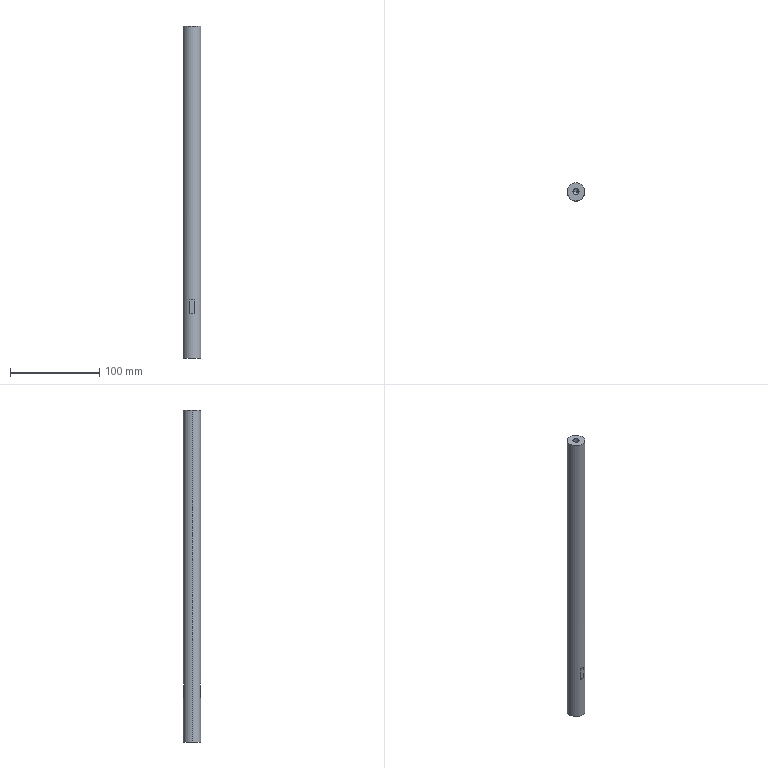Part | SolidWorks | features HoleWzd 2, Extrusion 1, ICE 1 | 1 solid | 18 faces | box 20 x 20 x 372 mm | volume 115321 mm3 | plane 8 | cylinder 6 | cone 4 | commonest cylinder face diameters 6.8 x4 20 x2
STEP:
#1=CARTESIAN_POINT('',(-3.4,0.,166.25));
#2=VERTEX_POINT('',#1);
#3=CARTESIAN_POINT('',(3.4,0.,166.25));
#4=VERTEX_POINT('',#3);
#5=CARTESIAN_POINT('',(0.,0.,166.25));
#6=DIRECTION('',(0.,0.,1.));
#7=DIRECTION('',(1.,0.,0.));
#8=AXIS2_PLACEMENT_3D('',#5,#6,#7);
#9=CIRCLE('',#8,3.4);
#10=EDGE_CURVE('',#2,#4,#9,.T.);
#11=ORIENTED_EDGE('',*,*,#10,.F.);
#12=CARTESIAN_POINT('',(-3.4,0.,186.));
#13=VERTEX_POINT('',#12);
#14=CARTESIAN_POINT('',(-3.4,0.,186.));
#15=DIRECTION('',(0.,0.,1.));
#16=VECTOR('',#15,1000.);
#17=LINE('',#14,#16);
#18=EDGE_CURVE('',#2,#13,#17,.T.);
#19=ORIENTED_EDGE('',*,*,#18,.T.);
#20=CARTESIAN_POINT('',(3.4,0.,186.));
#21=VERTEX_POINT('',#20);
#22=CARTESIAN_POINT('',(0.,0.,186.));
#23=DIRECTION('',(0.,0.,1.));
#24=DIRECTION('',(1.,0.,0.));
#25=AXIS2_PLACEMENT_3D('',#22,#23,#24);
#26=CIRCLE('',#25,3.4);
#27=EDGE_CURVE('',#13,#21,#26,.T.);
#28=ORIENTED_EDGE('',*,*,#27,.T.);
#29=CARTESIAN_POINT('',(3.4,0.,186.));
#30=DIRECTION('',(0.,0.,1.));
#31=VECTOR('',#30,1000.);
#32=LINE('',#29,#31);
#33=EDGE_CURVE('',#4,#21,#32,.T.);
#34=ORIENTED_EDGE('',*,*,#33,.F.);
#35=EDGE_LOOP('',(#11,#19,#28,#34));
#36=FACE_OUTER_BOUND('',#35,.T.);
#37=CARTESIAN_POINT('',(0.,0.,186.));
#38=DIRECTION('',(0.,0.,1.));
#39=DIRECTION('',(1.,0.,0.));
#40=AXIS2_PLACEMENT_3D('',#37,#38,#39);
#41=CYLINDRICAL_SURFACE('',#40,3.4);
#42=ADVANCED_FACE('',(#36),#41,.F.);
#43=CARTESIAN_POINT('',(0.,0.,164.207));
#44=VERTEX_POINT('',#43);
#45=CARTESIAN_POINT('',(3.4,0.,166.25));
#46=DIRECTION('',(0.8572,0.,0.515));
#47=VECTOR('',#46,1000.);
#48=LINE('',#45,#47);
#49=EDGE_CURVE('',#44,#4,#48,.T.);
#50=ORIENTED_EDGE('',*,*,#49,.F.);
#51=CARTESIAN_POINT('',(-3.4,0.,166.25));
#52=DIRECTION('',(-0.8572,0.,0.515));
#53=VECTOR('',#52,1000.);
#54=LINE('',#51,#53);
#55=EDGE_CURVE('',#44,#2,#54,.T.);
#56=ORIENTED_EDGE('',*,*,#55,.T.);
#57=ORIENTED_EDGE('',*,*,#10,.T.);
#58=EDGE_LOOP('',(#50,#56,#57));
#59=FACE_OUTER_BOUND('',#58,.T.);
#60=CARTESIAN_POINT('',(0.,0.,166.25));
#61=DIRECTION('',(0.,0.,1.));
#62=DIRECTION('',(1.,0.,0.));
#63=AXIS2_PLACEMENT_3D('',#60,#61,#62);
#64=CONICAL_SURFACE('',#63,3.4,1.03);
#65=ADVANCED_FACE('',(#59),#64,.F.);
#66=CARTESIAN_POINT('',(3.4,0.,-166.25));
#67=VERTEX_POINT('',#66);
#68=CARTESIAN_POINT('',(-3.4,0.,-166.25));
#69=VERTEX_POINT('',#68);
#70=CARTESIAN_POINT('',(0.,0.,-166.25));
#71=DIRECTION('',(0.,0.,-1.));
#72=DIRECTION('',(-1.,0.,0.));
#73=AXIS2_PLACEMENT_3D('',#70,#71,#72);
#74=CIRCLE('',#73,3.4);
#75=EDGE_CURVE('',#67,#69,#74,.T.);
#76=ORIENTED_EDGE('',*,*,#75,.F.);
#77=CARTESIAN_POINT('',(3.4,0.,-186.));
#78=VERTEX_POINT('',#77);
#79=CARTESIAN_POINT('',(3.4,0.,-186.));
#80=DIRECTION('',(0.,0.,-1.));
#81=VECTOR('',#80,1000.);
#82=LINE('',#79,#81);
#83=EDGE_CURVE('',#67,#78,#82,.T.);
#84=ORIENTED_EDGE('',*,*,#83,.T.);
#85=CARTESIAN_POINT('',(-3.4,0.,-186.));
#86=VERTEX_POINT('',#85);
#87=CARTESIAN_POINT('',(0.,0.,-186.));
#88=DIRECTION('',(0.,0.,-1.));
#89=DIRECTION('',(-1.,0.,0.));
#90=AXIS2_PLACEMENT_3D('',#87,#88,#89);
#91=CIRCLE('',#90,3.4);
#92=EDGE_CURVE('',#78,#86,#91,.T.);
#93=ORIENTED_EDGE('',*,*,#92,.T.);
#94=CARTESIAN_POINT('',(-3.4,0.,-186.));
#95=DIRECTION('',(0.,0.,-1.));
#96=VECTOR('',#95,1000.);
#97=LINE('',#94,#96);
#98=EDGE_CURVE('',#69,#86,#97,.T.);
#99=ORIENTED_EDGE('',*,*,#98,.F.);
#100=EDGE_LOOP('',(#76,#84,#93,#99));
#101=FACE_OUTER_BOUND('',#100,.T.);
#102=CARTESIAN_POINT('',(0.,0.,-186.));
#103=DIRECTION('',(0.,0.,-1.));
#104=DIRECTION('',(-1.,0.,0.));
#105=AXIS2_PLACEMENT_3D('',#102,#103,#104);
#106=CYLINDRICAL_SURFACE('',#105,3.4);
#107=ADVANCED_FACE('',(#101),#106,.F.);
#108=CARTESIAN_POINT('',(0.,0.,-164.207));
#109=VERTEX_POINT('',#108);
#110=CARTESIAN_POINT('',(-3.4,0.,-166.25));
#111=DIRECTION('',(-0.8572,0.,-0.515));
#112=VECTOR('',#111,1000.);
#113=LINE('',#110,#112);
#114=EDGE_CURVE('',#109,#69,#113,.T.);
#115=ORIENTED_EDGE('',*,*,#114,.F.);
#116=CARTESIAN_POINT('',(3.4,0.,-166.25));
#117=DIRECTION('',(0.8572,0.,-0.515));
#118=VECTOR('',#117,1000.);
#119=LINE('',#116,#118);
#120=EDGE_CURVE('',#109,#67,#119,.T.);
#121=ORIENTED_EDGE('',*,*,#120,.T.);
#122=ORIENTED_EDGE('',*,*,#75,.T.);
#123=EDGE_LOOP('',(#115,#121,#122));
#124=FACE_OUTER_BOUND('',#123,.T.);
#125=CARTESIAN_POINT('',(0.,0.,-166.25));
#126=DIRECTION('',(0.,0.,-1.));
#127=DIRECTION('',(-1.,0.,0.));
#128=AXIS2_PLACEMENT_3D('',#125,#126,#127);
#129=CONICAL_SURFACE('',#128,3.4,1.03);
#130=ADVANCED_FACE('',(#124),#129,.F.);
#131=CARTESIAN_POINT('',(-3.122,9.5,-136.));
#132=VERTEX_POINT('',#131);
#133=CARTESIAN_POINT('',(-3.122,9.5,-121.));
#134=VERTEX_POINT('',#133);
#135=CARTESIAN_POINT('',(-3.122,9.5,-136.));
#136=DIRECTION('',(0.,0.,1.));
#137=VECTOR('',#136,1000.);
#138=LINE('',#135,#137);
#139=EDGE_CURVE('',#132,#134,#138,.T.);
#140=ORIENTED_EDGE('',*,*,#139,.F.);
#141=CARTESIAN_POINT('',(3.122,9.5,-136.));
#142=VERTEX_POINT('',#141);
#143=CARTESIAN_POINT('',(0.,0.,-136.));
#144=DIRECTION('',(0.,0.,-1.));
#145=DIRECTION('',(-1.,0.,0.));
#146=AXIS2_PLACEMENT_3D('',#143,#144,#145);
#147=CIRCLE('',#146,10.);
#148=EDGE_CURVE('',#132,#142,#147,.T.);
#149=ORIENTED_EDGE('',*,*,#148,.T.);
#150=CARTESIAN_POINT('',(3.122,9.5,-121.));
#151=VERTEX_POINT('',#150);
#152=CARTESIAN_POINT('',(3.122,9.5,-136.));
#153=DIRECTION('',(0.,0.,1.));
#154=VECTOR('',#153,1000.);
#155=LINE('',#152,#154);
#156=EDGE_CURVE('',#142,#151,#155,.T.);
#157=ORIENTED_EDGE('',*,*,#156,.T.);
#158=CARTESIAN_POINT('',(0.,0.,-121.));
#159=DIRECTION('',(0.,0.,-1.));
#160=DIRECTION('',(-1.,0.,0.));
#161=AXIS2_PLACEMENT_3D('',#158,#159,#160);
#162=CIRCLE('',#161,10.);
#163=EDGE_CURVE('',#134,#151,#162,.T.);
#164=ORIENTED_EDGE('',*,*,#163,.F.);
#165=EDGE_LOOP('',(#140,#149,#157,#164));
#166=FACE_BOUND('',#165,.T.);
#167=CARTESIAN_POINT('',(10.,0.,186.));
#168=VERTEX_POINT('',#167);
#169=CARTESIAN_POINT('',(-10.,0.,186.));
#170=VERTEX_POINT('',#169);
#171=CARTESIAN_POINT('',(0.,0.,186.));
#172=DIRECTION('',(0.,0.,1.));
#173=DIRECTION('',(1.,0.,0.));
#174=AXIS2_PLACEMENT_3D('',#171,#172,#173);
#175=CIRCLE('',#174,10.);
#176=EDGE_CURVE('',#168,#170,#175,.T.);
#177=ORIENTED_EDGE('',*,*,#176,.F.);
#178=CARTESIAN_POINT('',(10.,0.,-186.));
#179=VERTEX_POINT('',#178);
#180=CARTESIAN_POINT('',(10.,0.,186.));
#181=DIRECTION('',(0.,0.,-1.));
#182=VECTOR('',#181,1000.);
#183=LINE('',#180,#182);
#184=EDGE_CURVE('',#168,#179,#183,.T.);
#185=ORIENTED_EDGE('',*,*,#184,.T.);
#186=CARTESIAN_POINT('',(-10.,0.,-186.));
#187=VERTEX_POINT('',#186);
#188=CARTESIAN_POINT('',(0.,0.,-186.));
#189=DIRECTION('',(0.,0.,1.));
#190=DIRECTION('',(1.,0.,0.));
#191=AXIS2_PLACEMENT_3D('',#188,#189,#190);
#192=CIRCLE('',#191,10.);
#193=EDGE_CURVE('',#179,#187,#192,.T.);
#194=ORIENTED_EDGE('',*,*,#193,.T.);
#195=CARTESIAN_POINT('',(-10.,0.,186.));
#196=DIRECTION('',(0.,0.,-1.));
#197=VECTOR('',#196,1000.);
#198=LINE('',#195,#197);
#199=EDGE_CURVE('',#170,#187,#198,.T.);
#200=ORIENTED_EDGE('',*,*,#199,.F.);
#201=EDGE_LOOP('',(#177,#185,#194,#200));
#202=FACE_OUTER_BOUND('',#201,.T.);
#203=CARTESIAN_POINT('',(0.,0.,186.));
#204=DIRECTION('',(0.,0.,-1.));
#205=DIRECTION('',(-1.,0.,0.));
#206=AXIS2_PLACEMENT_3D('',#203,#204,#205);
#207=CYLINDRICAL_SURFACE('',#206,10.);
#208=ADVANCED_FACE('',(#166,#202),#207,.T.);
#209=ORIENTED_EDGE('',*,*,#184,.F.);
#210=CARTESIAN_POINT('',(0.,0.,186.));
#211=DIRECTION('',(0.,0.,1.));
#212=DIRECTION('',(1.,0.,0.));
#213=AXIS2_PLACEMENT_3D('',#210,#211,#212);
#214=CIRCLE('',#213,10.);
#215=EDGE_CURVE('',#170,#168,#214,.T.);
#216=ORIENTED_EDGE('',*,*,#215,.F.);
#217=ORIENTED_EDGE('',*,*,#199,.T.);
#218=CARTESIAN_POINT('',(0.,0.,-186.));
#219=DIRECTION('',(0.,0.,1.));
#220=DIRECTION('',(1.,0.,0.));
#221=AXIS2_PLACEMENT_3D('',#218,#219,#220);
#222=CIRCLE('',#221,10.);
#223=EDGE_CURVE('',#187,#179,#222,.T.);
#224=ORIENTED_EDGE('',*,*,#223,.T.);
#225=EDGE_LOOP('',(#209,#216,#217,#224));
#226=FACE_OUTER_BOUND('',#225,.T.);
#227=CARTESIAN_POINT('',(3.122,-9.5,-136.));
#228=VERTEX_POINT('',#227);
#229=CARTESIAN_POINT('',(3.122,-9.5,-121.));
#230=VERTEX_POINT('',#229);
#231=CARTESIAN_POINT('',(3.122,-9.5,-136.));
#232=DIRECTION('',(0.,0.,1.));
#233=VECTOR('',#232,1000.);
#234=LINE('',#231,#233);
#235=EDGE_CURVE('',#228,#230,#234,.T.);
#236=ORIENTED_EDGE('',*,*,#235,.F.);
#237=CARTESIAN_POINT('',(-3.122,-9.5,-136.));
#238=VERTEX_POINT('',#237);
#239=CARTESIAN_POINT('',(0.,0.,-136.));
#240=DIRECTION('',(0.,0.,-1.));
#241=DIRECTION('',(-1.,0.,0.));
#242=AXIS2_PLACEMENT_3D('',#239,#240,#241);
#243=CIRCLE('',#242,10.);
#244=EDGE_CURVE('',#228,#238,#243,.T.);
#245=ORIENTED_EDGE('',*,*,#244,.T.);
#246=CARTESIAN_POINT('',(-3.122,-9.5,-121.));
#247=VERTEX_POINT('',#246);
#248=CARTESIAN_POINT('',(-3.122,-9.5,-136.));
#249=DIRECTION('',(0.,0.,1.));
#250=VECTOR('',#249,1000.);
#251=LINE('',#248,#250);
#252=EDGE_CURVE('',#238,#247,#251,.T.);
#253=ORIENTED_EDGE('',*,*,#252,.T.);
#254=CARTESIAN_POINT('',(0.,0.,-121.));
#255=DIRECTION('',(0.,0.,-1.));
#256=DIRECTION('',(-1.,0.,0.));
#257=AXIS2_PLACEMENT_3D('',#254,#255,#256);
#258=CIRCLE('',#257,10.);
#259=EDGE_CURVE('',#230,#247,#258,.T.);
#260=ORIENTED_EDGE('',*,*,#259,.F.);
#261=EDGE_LOOP('',(#236,#245,#253,#260));
#262=FACE_BOUND('',#261,.T.);
#263=CARTESIAN_POINT('',(0.,0.,186.));
#264=DIRECTION('',(0.,0.,-1.));
#265=DIRECTION('',(-1.,0.,0.));
#266=AXIS2_PLACEMENT_3D('',#263,#264,#265);
#267=CYLINDRICAL_SURFACE('',#266,10.);
#268=ADVANCED_FACE('',(#226,#262),#267,.T.);
#269=CARTESIAN_POINT('',(0.,0.,186.));
#270=DIRECTION('',(0.,0.,1.));
#271=DIRECTION('',(1.,0.,0.));
#272=AXIS2_PLACEMENT_3D('',#269,#270,#271);
#273=CIRCLE('',#272,3.4);
#274=EDGE_CURVE('',#21,#13,#273,.T.);
#275=ORIENTED_EDGE('',*,*,#274,.F.);
#276=ORIENTED_EDGE('',*,*,#27,.F.);
#277=EDGE_LOOP('',(#275,#276));
#278=FACE_BOUND('',#277,.T.);
#279=ORIENTED_EDGE('',*,*,#215,.T.);
#280=ORIENTED_EDGE('',*,*,#176,.T.);
#281=EDGE_LOOP('',(#279,#280));
#282=FACE_OUTER_BOUND('',#281,.T.);
#283=CARTESIAN_POINT('',(0.,0.,186.));
#284=DIRECTION('',(0.,0.,1.));
#285=DIRECTION('',(1.,0.,0.));
#286=AXIS2_PLACEMENT_3D('',#283,#284,#285);
#287=PLANE('',#286);
#288=ADVANCED_FACE('',(#278,#282),#287,.T.);
#289=CARTESIAN_POINT('',(0.,0.,-186.));
#290=DIRECTION('',(0.,0.,-1.));
#291=DIRECTION('',(-1.,0.,0.));
#292=AXIS2_PLACEMENT_3D('',#289,#290,#291);
#293=CIRCLE('',#292,3.4);
#294=EDGE_CURVE('',#86,#78,#293,.T.);
#295=ORIENTED_EDGE('',*,*,#294,.F.);
#296=ORIENTED_EDGE('',*,*,#92,.F.);
#297=EDGE_LOOP('',(#295,#296));
#298=FACE_BOUND('',#297,.T.);
#299=ORIENTED_EDGE('',*,*,#223,.F.);
#300=ORIENTED_EDGE('',*,*,#193,.F.);
#301=EDGE_LOOP('',(#299,#300));
#302=FACE_OUTER_BOUND('',#301,.T.);
#303=CARTESIAN_POINT('',(0.,0.,-186.));
#304=DIRECTION('',(0.,0.,1.));
#305=DIRECTION('',(1.,0.,0.));
#306=AXIS2_PLACEMENT_3D('',#303,#304,#305);
#307=PLANE('',#306);
#308=ADVANCED_FACE('',(#298,#302),#307,.F.);
#309=CARTESIAN_POINT('',(3.122,-9.5,-121.));
#310=DIRECTION('',(1.,0.,0.));
#311=VECTOR('',#310,1000.);
#312=LINE('',#309,#311);
#313=EDGE_CURVE('',#247,#230,#312,.T.);
#314=ORIENTED_EDGE('',*,*,#313,.F.);
#315=ORIENTED_EDGE('',*,*,#252,.F.);
#316=CARTESIAN_POINT('',(3.122,-9.5,-136.));
#317=DIRECTION('',(1.,0.,0.));
#318=VECTOR('',#317,1000.);
#319=LINE('',#316,#318);
#320=EDGE_CURVE('',#238,#228,#319,.T.);
#321=ORIENTED_EDGE('',*,*,#320,.T.);
#322=ORIENTED_EDGE('',*,*,#235,.T.);
#323=EDGE_LOOP('',(#314,#315,#321,#322));
#324=FACE_OUTER_BOUND('',#323,.T.);
#325=CARTESIAN_POINT('',(3.122,-9.5,-136.));
#326=DIRECTION('',(0.,-1.,0.));
#327=DIRECTION('',(0.,0.,-1.));
#328=AXIS2_PLACEMENT_3D('',#325,#326,#327);
#329=PLANE('',#328);
#330=ADVANCED_FACE('',(#324),#329,.T.);
#331=ORIENTED_EDGE('',*,*,#244,.F.);
#332=ORIENTED_EDGE('',*,*,#320,.F.);
#333=EDGE_LOOP('',(#331,#332));
#334=FACE_OUTER_BOUND('',#333,.T.);
#335=CARTESIAN_POINT('',(0.,0.,-136.));
#336=DIRECTION('',(0.,0.,-1.));
#337=DIRECTION('',(-1.,0.,0.));
#338=AXIS2_PLACEMENT_3D('',#335,#336,#337);
#339=PLANE('',#338);
#340=ADVANCED_FACE('',(#334),#339,.F.);
#341=ORIENTED_EDGE('',*,*,#259,.T.);
#342=ORIENTED_EDGE('',*,*,#313,.T.);
#343=EDGE_LOOP('',(#341,#342));
#344=FACE_OUTER_BOUND('',#343,.T.);
#345=CARTESIAN_POINT('',(0.,0.,-121.));
#346=DIRECTION('',(0.,0.,-1.));
#347=DIRECTION('',(-1.,0.,0.));
#348=AXIS2_PLACEMENT_3D('',#345,#346,#347);
#349=PLANE('',#348);
#350=ADVANCED_FACE('',(#344),#349,.T.);
#351=CARTESIAN_POINT('',(3.122,9.5,-121.));
#352=DIRECTION('',(-1.,0.,0.));
#353=VECTOR('',#352,1000.);
#354=LINE('',#351,#353);
#355=EDGE_CURVE('',#151,#134,#354,.T.);
#356=ORIENTED_EDGE('',*,*,#355,.F.);
#357=ORIENTED_EDGE('',*,*,#156,.F.);
#358=CARTESIAN_POINT('',(3.122,9.5,-136.));
#359=DIRECTION('',(-1.,0.,0.));
#360=VECTOR('',#359,1000.);
#361=LINE('',#358,#360);
#362=EDGE_CURVE('',#142,#132,#361,.T.);
#363=ORIENTED_EDGE('',*,*,#362,.T.);
#364=ORIENTED_EDGE('',*,*,#139,.T.);
#365=EDGE_LOOP('',(#356,#357,#363,#364));
#366=FACE_OUTER_BOUND('',#365,.T.);
#367=CARTESIAN_POINT('',(3.122,9.5,-136.));
#368=DIRECTION('',(0.,1.,0.));
#369=DIRECTION('',(0.,0.,1.));
#370=AXIS2_PLACEMENT_3D('',#367,#368,#369);
#371=PLANE('',#370);
#372=ADVANCED_FACE('',(#366),#371,.T.);
#373=ORIENTED_EDGE('',*,*,#148,.F.);
#374=ORIENTED_EDGE('',*,*,#362,.F.);
#375=EDGE_LOOP('',(#373,#374));
#376=FACE_OUTER_BOUND('',#375,.T.);
#377=CARTESIAN_POINT('',(0.,0.,-136.));
#378=DIRECTION('',(0.,0.,-1.));
#379=DIRECTION('',(-1.,0.,0.));
#380=AXIS2_PLACEMENT_3D('',#377,#378,#379);
#381=PLANE('',#380);
#382=ADVANCED_FACE('',(#376),#381,.F.);
#383=ORIENTED_EDGE('',*,*,#163,.T.);
#384=ORIENTED_EDGE('',*,*,#355,.T.);
#385=EDGE_LOOP('',(#383,#384));
#386=FACE_OUTER_BOUND('',#385,.T.);
#387=CARTESIAN_POINT('',(0.,0.,-121.));
#388=DIRECTION('',(0.,0.,-1.));
#389=DIRECTION('',(-1.,0.,0.));
#390=AXIS2_PLACEMENT_3D('',#387,#388,#389);
#391=PLANE('',#390);
#392=ADVANCED_FACE('',(#386),#391,.T.);
#393=ORIENTED_EDGE('',*,*,#120,.F.);
#394=ORIENTED_EDGE('',*,*,#114,.T.);
#395=CARTESIAN_POINT('',(0.,0.,-166.25));
#396=DIRECTION('',(0.,0.,-1.));
#397=DIRECTION('',(-1.,0.,0.));
#398=AXIS2_PLACEMENT_3D('',#395,#396,#397);
#399=CIRCLE('',#398,3.4);
#400=EDGE_CURVE('',#69,#67,#399,.T.);
#401=ORIENTED_EDGE('',*,*,#400,.T.);
#402=EDGE_LOOP('',(#393,#394,#401));
#403=FACE_OUTER_BOUND('',#402,.T.);
#404=CARTESIAN_POINT('',(0.,0.,-166.25));
#405=DIRECTION('',(0.,0.,-1.));
#406=DIRECTION('',(-1.,0.,0.));
#407=AXIS2_PLACEMENT_3D('',#404,#405,#406);
#408=CONICAL_SURFACE('',#407,3.4,1.03);
#409=ADVANCED_FACE('',(#403),#408,.F.);
#410=ORIENTED_EDGE('',*,*,#83,.F.);
#411=ORIENTED_EDGE('',*,*,#400,.F.);
#412=ORIENTED_EDGE('',*,*,#98,.T.);
#413=ORIENTED_EDGE('',*,*,#294,.T.);
#414=EDGE_LOOP('',(#410,#411,#412,#413));
#415=FACE_OUTER_BOUND('',#414,.T.);
#416=CARTESIAN_POINT('',(0.,0.,-186.));
#417=DIRECTION('',(0.,0.,-1.));
#418=DIRECTION('',(-1.,0.,0.));
#419=AXIS2_PLACEMENT_3D('',#416,#417,#418);
#420=CYLINDRICAL_SURFACE('',#419,3.4);
#421=ADVANCED_FACE('',(#415),#420,.F.);
#422=ORIENTED_EDGE('',*,*,#55,.F.);
#423=ORIENTED_EDGE('',*,*,#49,.T.);
#424=CARTESIAN_POINT('',(0.,0.,166.25));
#425=DIRECTION('',(0.,0.,1.));
#426=DIRECTION('',(1.,0.,0.));
#427=AXIS2_PLACEMENT_3D('',#424,#425,#426);
#428=CIRCLE('',#427,3.4);
#429=EDGE_CURVE('',#4,#2,#428,.T.);
#430=ORIENTED_EDGE('',*,*,#429,.T.);
#431=EDGE_LOOP('',(#422,#423,#430));
#432=FACE_OUTER_BOUND('',#431,.T.);
#433=CARTESIAN_POINT('',(0.,0.,166.25));
#434=DIRECTION('',(0.,0.,1.));
#435=DIRECTION('',(1.,0.,0.));
#436=AXIS2_PLACEMENT_3D('',#433,#434,#435);
#437=CONICAL_SURFACE('',#436,3.4,1.03);
#438=ADVANCED_FACE('',(#432),#437,.F.);
#439=ORIENTED_EDGE('',*,*,#18,.F.);
#440=ORIENTED_EDGE('',*,*,#429,.F.);
#441=ORIENTED_EDGE('',*,*,#33,.T.);
#442=ORIENTED_EDGE('',*,*,#274,.T.);
#443=EDGE_LOOP('',(#439,#440,#441,#442));
#444=FACE_OUTER_BOUND('',#443,.T.);
#445=CARTESIAN_POINT('',(0.,0.,186.));
#446=DIRECTION('',(0.,0.,1.));
#447=DIRECTION('',(1.,0.,0.));
#448=AXIS2_PLACEMENT_3D('',#445,#446,#447);
#449=CYLINDRICAL_SURFACE('',#448,3.4);
#450=ADVANCED_FACE('',(#444),#449,.F.);
#451=CLOSED_SHELL('',(#42,#65,#107,#130,#208,#268,#288,#308,#330,#340,#350,#372,#382,#392,#409,#421,#438,#450));
#452=MANIFOLD_SOLID_BREP('',#451);
#453=CARTESIAN_POINT('',(0.,0.,0.));
#454=DIRECTION('',(0.,0.,1.));
#455=DIRECTION('',(1.,0.,0.));
#456=AXIS2_PLACEMENT_3D('',#453,#454,#455);
#457=(LENGTH_UNIT()NAMED_UNIT(*)SI_UNIT(.MILLI.,.METRE.));
#458=UNCERTAINTY_MEASURE_WITH_UNIT(LENGTH_MEASURE(0.00001),#457,'','');
#459=(NAMED_UNIT(*)PLANE_ANGLE_UNIT()SI_UNIT($,.RADIAN.));
#460=(NAMED_UNIT(*)SI_UNIT($,.STERADIAN.)SOLID_ANGLE_UNIT());
#461=(GEOMETRIC_REPRESENTATION_CONTEXT(3)GLOBAL_UNCERTAINTY_ASSIGNED_CONTEXT((#458))GLOBAL_UNIT_ASSIGNED_CONTEXT((#457,#459,#460))REPRESENTATION_CONTEXT('',''));
#462=ADVANCED_BREP_SHAPE_REPRESENTATION('',(#452,#456),#461);